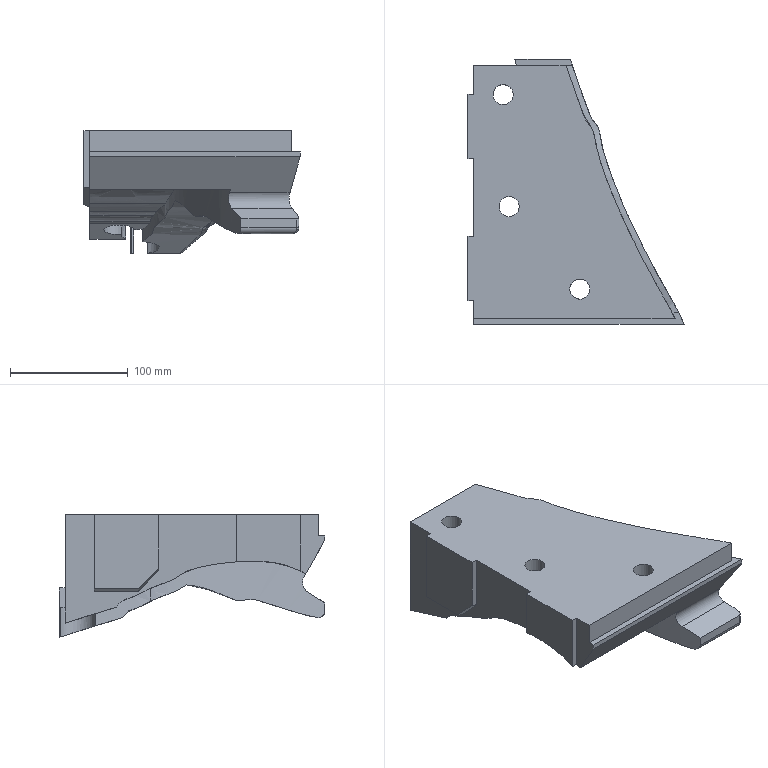Part | NX | features solid 2 | 1 solid | 65 faces | volume 1584811 mm3 | spline 27 | plane 26 | cylinder 12 | commonest cylinder face diameters 17 x3 26 x3 32 x3 4 x1 10 x1 20 x1